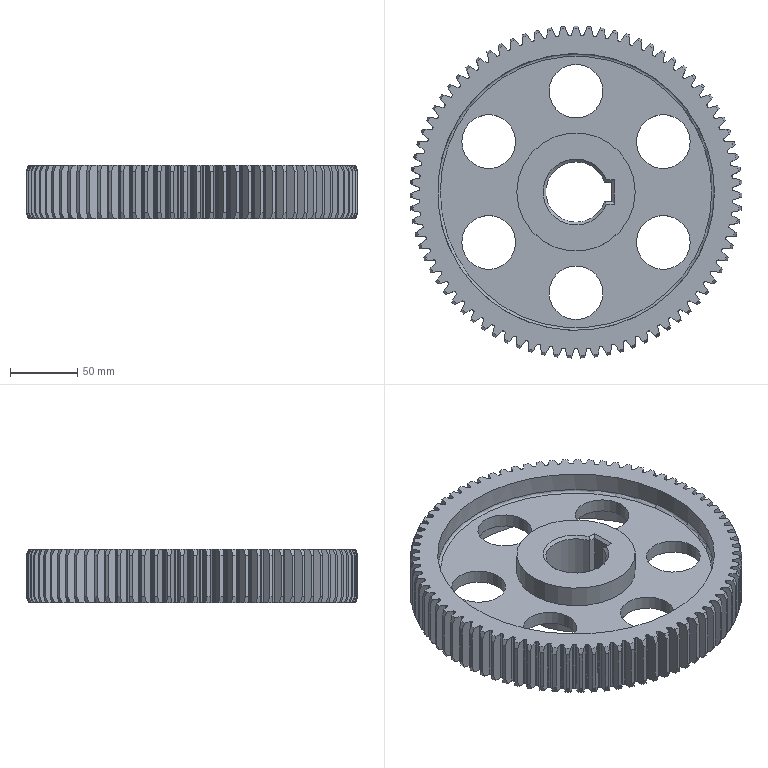Part | NX | features BREP 79, META 79, DATUM_CSYS 7, SKETCH 6, EXTRUDE 5, CPROJ 2, BLEND 1, CHAMFER 1, CYLINDER 1, FSET 1, SWP104 1 | 1 solid | 662 faces | box 247.038 x 246.995 x 40 mm | volume 857249 mm3 | spline 395 | cone 160 | cylinder 90 | plane 15 | torus 2 | commonest cylinder face diameters 233.325 x79 40 x6 88 x2 206 x2 45 x1